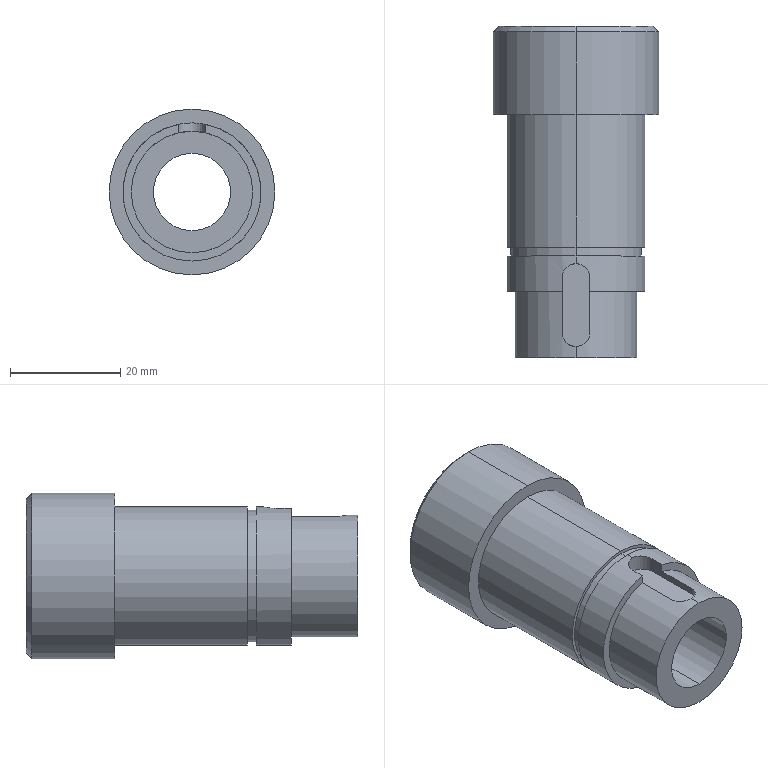Part | SolidWorks | features ICE 3, Chamfer 1, HoleWzd 1, RevCut 1, Revolution 1 | 1 solid | 28 faces | box 30 x 60 x 30 mm | volume 20081 mm3 | cylinder 16 | plane 10 | cone 2 | commonest cylinder face diameters 25 x4 5 x2 14 x2 18 x2 22 x2 23.8 x2
STEP:
#1=CARTESIAN_POINT('',(2.5,4.5,10.712));
#2=VERTEX_POINT('',#1);
#3=CARTESIAN_POINT('',(0.,2.,11.));
#4=VERTEX_POINT('',#3);
#5=CARTESIAN_POINT('',(2.5,4.5,10.712));
#6=CARTESIAN_POINT('',(2.5,4.334,10.712));
#7=CARTESIAN_POINT('',(2.484,4.171,10.716));
#8=CARTESIAN_POINT('',(2.42,3.851,10.731));
#9=CARTESIAN_POINT('',(2.371,3.692,10.742));
#10=CARTESIAN_POINT('',(2.246,3.389,10.769));
#11=CARTESIAN_POINT('',(2.169,3.246,10.784));
#12=CARTESIAN_POINT('',(1.987,2.974,10.819));
#13=CARTESIAN_POINT('',(1.882,2.846,10.838));
#14=CARTESIAN_POINT('',(1.537,2.502,10.895));
#15=CARTESIAN_POINT('',(1.259,2.316,10.932));
#16=CARTESIAN_POINT('',(0.8077,2.128,10.971));
#17=CARTESIAN_POINT('',(0.6494,2.08,10.982));
#18=CARTESIAN_POINT('',(0.3264,2.016,10.996));
#19=CARTESIAN_POINT('',(0.1637,2.,11.));
#20=CARTESIAN_POINT('',(0.,2.,11.));
#21=B_SPLINE_CURVE_WITH_KNOTS('',3,(#5,#6,#7,#8,#9,#10,#11,#12,#13,#14,#15,#16,#17,#18,#19,#20),.UNSPECIFIED.,.F.,.F.,(4,2,2,2,2,2,2,4),(0.,0.0004902,0.0009805,0.001471,0.001961,0.002941,0.003432,0.003922),.UNSPECIFIED.);
#22=EDGE_CURVE('',#2,#4,#21,.T.);
#23=ORIENTED_EDGE('',*,*,#22,.T.);
#24=CARTESIAN_POINT('',(0.,0.,11.));
#25=VERTEX_POINT('',#24);
#26=CARTESIAN_POINT('',(0.,12.,11.));
#27=DIRECTION('',(0.,-1.,0.));
#28=VECTOR('',#27,1000.);
#29=LINE('',#26,#28);
#30=EDGE_CURVE('',#4,#25,#29,.T.);
#31=ORIENTED_EDGE('',*,*,#30,.T.);
#32=CARTESIAN_POINT('',(0.,0.,-11.));
#33=VERTEX_POINT('',#32);
#34=CARTESIAN_POINT('',(0.,0.,0.));
#35=DIRECTION('',(0.,-1.,0.));
#36=DIRECTION('',(0.,0.,-1.));
#37=AXIS2_PLACEMENT_3D('',#34,#35,#36);
#38=CIRCLE('',#37,11.);
#39=EDGE_CURVE('',#33,#25,#38,.T.);
#40=ORIENTED_EDGE('',*,*,#39,.F.);
#41=CARTESIAN_POINT('',(0.,12.,-11.));
#42=VERTEX_POINT('',#41);
#43=CARTESIAN_POINT('',(0.,12.,-11.));
#44=DIRECTION('',(0.,-1.,0.));
#45=VECTOR('',#44,1000.);
#46=LINE('',#43,#45);
#47=EDGE_CURVE('',#42,#33,#46,.T.);
#48=ORIENTED_EDGE('',*,*,#47,.F.);
#49=CARTESIAN_POINT('',(2.5,12.,10.712));
#50=VERTEX_POINT('',#49);
#51=CARTESIAN_POINT('',(0.,12.,0.));
#52=DIRECTION('',(0.,-1.,0.));
#53=DIRECTION('',(0.,0.,-1.));
#54=AXIS2_PLACEMENT_3D('',#51,#52,#53);
#55=CIRCLE('',#54,11.);
#56=EDGE_CURVE('',#42,#50,#55,.T.);
#57=ORIENTED_EDGE('',*,*,#56,.T.);
#58=CARTESIAN_POINT('',(2.5,12.,10.712));
#59=DIRECTION('',(0.,-1.,0.));
#60=VECTOR('',#59,1000.);
#61=LINE('',#58,#60);
#62=EDGE_CURVE('',#50,#2,#61,.T.);
#63=ORIENTED_EDGE('',*,*,#62,.T.);
#64=EDGE_LOOP('',(#23,#31,#40,#48,#57,#63));
#65=FACE_OUTER_BOUND('',#64,.T.);
#66=CARTESIAN_POINT('',(0.,12.,0.));
#67=DIRECTION('',(0.,-1.,0.));
#68=DIRECTION('',(0.,0.,-1.));
#69=AXIS2_PLACEMENT_3D('',#66,#67,#68);
#70=CYLINDRICAL_SURFACE('',#69,11.);
#71=ADVANCED_FACE('',(#65),#70,.T.);
#72=CARTESIAN_POINT('',(0.,60.,14.));
#73=VERTEX_POINT('',#72);
#74=CARTESIAN_POINT('',(0.,60.,-14.));
#75=VERTEX_POINT('',#74);
#76=CARTESIAN_POINT('',(0.,60.,0.));
#77=DIRECTION('',(0.,1.,0.));
#78=DIRECTION('',(0.,0.,1.));
#79=AXIS2_PLACEMENT_3D('',#76,#77,#78);
#80=CIRCLE('',#79,14.);
#81=EDGE_CURVE('',#73,#75,#80,.T.);
#82=ORIENTED_EDGE('',*,*,#81,.F.);
#83=CARTESIAN_POINT('',(0.,59.,15.));
#84=VERTEX_POINT('',#83);
#85=CARTESIAN_POINT('',(0.,59.,15.));
#86=DIRECTION('',(0.,-0.7071,0.7071));
#87=VECTOR('',#86,1000.);
#88=LINE('',#85,#87);
#89=EDGE_CURVE('',#73,#84,#88,.T.);
#90=ORIENTED_EDGE('',*,*,#89,.T.);
#91=CARTESIAN_POINT('',(0.,59.,-15.));
#92=VERTEX_POINT('',#91);
#93=CARTESIAN_POINT('',(0.,59.,0.));
#94=DIRECTION('',(0.,-1.,0.));
#95=DIRECTION('',(0.,0.,1.));
#96=AXIS2_PLACEMENT_3D('',#93,#94,#95);
#97=CIRCLE('',#96,15.);
#98=EDGE_CURVE('',#92,#84,#97,.T.);
#99=ORIENTED_EDGE('',*,*,#98,.F.);
#100=CARTESIAN_POINT('',(0.,59.,-15.));
#101=DIRECTION('',(0.,-0.7071,-0.7071));
#102=VECTOR('',#101,1000.);
#103=LINE('',#100,#102);
#104=EDGE_CURVE('',#75,#92,#103,.T.);
#105=ORIENTED_EDGE('',*,*,#104,.F.);
#106=EDGE_LOOP('',(#82,#90,#99,#105));
#107=FACE_OUTER_BOUND('',#106,.T.);
#108=CARTESIAN_POINT('',(0.,59.,0.));
#109=DIRECTION('',(0.,-1.,0.));
#110=DIRECTION('',(0.,0.,-1.));
#111=AXIS2_PLACEMENT_3D('',#108,#109,#110);
#112=CONICAL_SURFACE('',#111,15.,0.7854);
#113=ADVANCED_FACE('',(#107),#112,.T.);
#114=CARTESIAN_POINT('',(0.,40.,-7.));
#115=VERTEX_POINT('',#114);
#116=CARTESIAN_POINT('',(0.,40.,7.));
#117=VERTEX_POINT('',#116);
#118=CARTESIAN_POINT('',(0.,40.,0.));
#119=DIRECTION('',(0.,1.,0.));
#120=DIRECTION('',(0.,0.,1.));
#121=AXIS2_PLACEMENT_3D('',#118,#119,#120);
#122=CIRCLE('',#121,7.);
#123=EDGE_CURVE('',#115,#117,#122,.T.);
#124=ORIENTED_EDGE('',*,*,#123,.T.);
#125=CARTESIAN_POINT('',(0.,0.,7.));
#126=VERTEX_POINT('',#125);
#127=CARTESIAN_POINT('',(0.,0.,7.));
#128=DIRECTION('',(0.,-1.,0.));
#129=VECTOR('',#128,1000.);
#130=LINE('',#127,#129);
#131=EDGE_CURVE('',#117,#126,#130,.T.);
#132=ORIENTED_EDGE('',*,*,#131,.T.);
#133=CARTESIAN_POINT('',(0.,0.,-7.));
#134=VERTEX_POINT('',#133);
#135=CARTESIAN_POINT('',(0.,0.,0.));
#136=DIRECTION('',(0.,-1.,0.));
#137=DIRECTION('',(0.,0.,-1.));
#138=AXIS2_PLACEMENT_3D('',#135,#136,#137);
#139=CIRCLE('',#138,7.);
#140=EDGE_CURVE('',#126,#134,#139,.T.);
#141=ORIENTED_EDGE('',*,*,#140,.T.);
#142=CARTESIAN_POINT('',(0.,0.,-7.));
#143=DIRECTION('',(0.,-1.,0.));
#144=VECTOR('',#143,1000.);
#145=LINE('',#142,#144);
#146=EDGE_CURVE('',#115,#134,#145,.T.);
#147=ORIENTED_EDGE('',*,*,#146,.F.);
#148=EDGE_LOOP('',(#124,#132,#141,#147));
#149=FACE_OUTER_BOUND('',#148,.T.);
#150=CARTESIAN_POINT('',(0.,0.,0.));
#151=DIRECTION('',(0.,-1.,0.));
#152=DIRECTION('',(0.,0.,-1.));
#153=AXIS2_PLACEMENT_3D('',#150,#151,#152);
#154=CYLINDRICAL_SURFACE('',#153,7.);
#155=ADVANCED_FACE('',(#149),#154,.F.);
#156=CARTESIAN_POINT('',(0.,40.,-9.));
#157=VERTEX_POINT('',#156);
#158=CARTESIAN_POINT('',(0.,40.,9.));
#159=VERTEX_POINT('',#158);
#160=CARTESIAN_POINT('',(0.,40.,0.));
#161=DIRECTION('',(0.,1.,0.));
#162=DIRECTION('',(0.,0.,1.));
#163=AXIS2_PLACEMENT_3D('',#160,#161,#162);
#164=CIRCLE('',#163,9.);
#165=EDGE_CURVE('',#157,#159,#164,.T.);
#166=ORIENTED_EDGE('',*,*,#165,.F.);
#167=CARTESIAN_POINT('',(0.,60.,-9.));
#168=VERTEX_POINT('',#167);
#169=CARTESIAN_POINT('',(0.,40.,-9.));
#170=DIRECTION('',(0.,1.,0.));
#171=VECTOR('',#170,1000.);
#172=LINE('',#169,#171);
#173=EDGE_CURVE('',#157,#168,#172,.T.);
#174=ORIENTED_EDGE('',*,*,#173,.T.);
#175=CARTESIAN_POINT('',(0.,60.,9.));
#176=VERTEX_POINT('',#175);
#177=CARTESIAN_POINT('',(0.,60.,0.));
#178=DIRECTION('',(0.,1.,0.));
#179=DIRECTION('',(0.,0.,1.));
#180=AXIS2_PLACEMENT_3D('',#177,#178,#179);
#181=CIRCLE('',#180,9.);
#182=EDGE_CURVE('',#168,#176,#181,.T.);
#183=ORIENTED_EDGE('',*,*,#182,.T.);
#184=CARTESIAN_POINT('',(0.,40.,9.));
#185=DIRECTION('',(0.,1.,0.));
#186=VECTOR('',#185,1000.);
#187=LINE('',#184,#186);
#188=EDGE_CURVE('',#159,#176,#187,.T.);
#189=ORIENTED_EDGE('',*,*,#188,.F.);
#190=EDGE_LOOP('',(#166,#174,#183,#189));
#191=FACE_OUTER_BOUND('',#190,.T.);
#192=CARTESIAN_POINT('',(0.,40.,0.));
#193=DIRECTION('',(0.,1.,0.));
#194=DIRECTION('',(0.,0.,1.));
#195=AXIS2_PLACEMENT_3D('',#192,#193,#194);
#196=CYLINDRICAL_SURFACE('',#195,9.);
#197=ADVANCED_FACE('',(#191),#196,.F.);
#198=CARTESIAN_POINT('',(0.,20.,-11.9));
#199=VERTEX_POINT('',#198);
#200=CARTESIAN_POINT('',(0.,20.,11.9));
#201=VERTEX_POINT('',#200);
#202=CARTESIAN_POINT('',(0.,20.,0.));
#203=DIRECTION('',(0.,-1.,0.));
#204=DIRECTION('',(0.,0.,-1.));
#205=AXIS2_PLACEMENT_3D('',#202,#203,#204);
#206=CIRCLE('',#205,11.9);
#207=EDGE_CURVE('',#199,#201,#206,.T.);
#208=ORIENTED_EDGE('',*,*,#207,.T.);
#209=CARTESIAN_POINT('',(0.,18.4,11.9));
#210=VERTEX_POINT('',#209);
#211=CARTESIAN_POINT('',(0.,0.,11.9));
#212=DIRECTION('',(0.,-1.,0.));
#213=VECTOR('',#212,1000.);
#214=LINE('',#211,#213);
#215=EDGE_CURVE('',#201,#210,#214,.T.);
#216=ORIENTED_EDGE('',*,*,#215,.T.);
#217=CARTESIAN_POINT('',(0.,18.4,-11.9));
#218=VERTEX_POINT('',#217);
#219=CARTESIAN_POINT('',(0.,18.4,0.));
#220=DIRECTION('',(0.,-1.,0.));
#221=DIRECTION('',(0.,0.,-1.));
#222=AXIS2_PLACEMENT_3D('',#219,#220,#221);
#223=CIRCLE('',#222,11.9);
#224=EDGE_CURVE('',#218,#210,#223,.T.);
#225=ORIENTED_EDGE('',*,*,#224,.F.);
#226=CARTESIAN_POINT('',(0.,0.,-11.9));
#227=DIRECTION('',(0.,-1.,0.));
#228=VECTOR('',#227,1000.);
#229=LINE('',#226,#228);
#230=EDGE_CURVE('',#199,#218,#229,.T.);
#231=ORIENTED_EDGE('',*,*,#230,.F.);
#232=EDGE_LOOP('',(#208,#216,#225,#231));
#233=FACE_OUTER_BOUND('',#232,.T.);
#234=CARTESIAN_POINT('',(0.,0.,0.));
#235=DIRECTION('',(0.,-1.,0.));
#236=DIRECTION('',(0.,0.,-1.));
#237=AXIS2_PLACEMENT_3D('',#234,#235,#236);
#238=CYLINDRICAL_SURFACE('',#237,11.9);
#239=ADVANCED_FACE('',(#233),#238,.T.);
#240=ORIENTED_EDGE('',*,*,#98,.T.);
#241=CARTESIAN_POINT('',(0.,44.,15.));
#242=VERTEX_POINT('',#241);
#243=CARTESIAN_POINT('',(0.,0.,15.));
#244=DIRECTION('',(0.,-1.,0.));
#245=VECTOR('',#244,1000.);
#246=LINE('',#243,#245);
#247=EDGE_CURVE('',#84,#242,#246,.T.);
#248=ORIENTED_EDGE('',*,*,#247,.T.);
#249=CARTESIAN_POINT('',(0.,44.,-15.));
#250=VERTEX_POINT('',#249);
#251=CARTESIAN_POINT('',(0.,44.,0.));
#252=DIRECTION('',(0.,-1.,0.));
#253=DIRECTION('',(0.,0.,-1.));
#254=AXIS2_PLACEMENT_3D('',#251,#252,#253);
#255=CIRCLE('',#254,15.);
#256=EDGE_CURVE('',#250,#242,#255,.T.);
#257=ORIENTED_EDGE('',*,*,#256,.F.);
#258=CARTESIAN_POINT('',(0.,0.,-15.));
#259=DIRECTION('',(0.,-1.,0.));
#260=VECTOR('',#259,1000.);
#261=LINE('',#258,#260);
#262=EDGE_CURVE('',#92,#250,#261,.T.);
#263=ORIENTED_EDGE('',*,*,#262,.F.);
#264=EDGE_LOOP('',(#240,#248,#257,#263));
#265=FACE_OUTER_BOUND('',#264,.T.);
#266=CARTESIAN_POINT('',(0.,0.,0.));
#267=DIRECTION('',(0.,-1.,0.));
#268=DIRECTION('',(0.,0.,-1.));
#269=AXIS2_PLACEMENT_3D('',#266,#267,#268);
#270=CYLINDRICAL_SURFACE('',#269,15.);
#271=ADVANCED_FACE('',(#265),#270,.T.);
#272=CARTESIAN_POINT('',(0.,44.,-12.5));
#273=VERTEX_POINT('',#272);
#274=CARTESIAN_POINT('',(0.,44.,12.5));
#275=VERTEX_POINT('',#274);
#276=CARTESIAN_POINT('',(0.,44.,0.));
#277=DIRECTION('',(0.,-1.,0.));
#278=DIRECTION('',(0.,0.,-1.));
#279=AXIS2_PLACEMENT_3D('',#276,#277,#278);
#280=CIRCLE('',#279,12.5);
#281=EDGE_CURVE('',#273,#275,#280,.T.);
#282=ORIENTED_EDGE('',*,*,#281,.T.);
#283=CARTESIAN_POINT('',(0.,20.,12.5));
#284=VERTEX_POINT('',#283);
#285=CARTESIAN_POINT('',(0.,0.,12.5));
#286=DIRECTION('',(0.,-1.,0.));
#287=VECTOR('',#286,1000.);
#288=LINE('',#285,#287);
#289=EDGE_CURVE('',#275,#284,#288,.T.);
#290=ORIENTED_EDGE('',*,*,#289,.T.);
#291=CARTESIAN_POINT('',(0.,20.,-12.5));
#292=VERTEX_POINT('',#291);
#293=CARTESIAN_POINT('',(0.,20.,0.));
#294=DIRECTION('',(0.,1.,0.));
#295=DIRECTION('',(0.,0.,-1.));
#296=AXIS2_PLACEMENT_3D('',#293,#294,#295);
#297=CIRCLE('',#296,12.5);
#298=EDGE_CURVE('',#284,#292,#297,.T.);
#299=ORIENTED_EDGE('',*,*,#298,.T.);
#300=CARTESIAN_POINT('',(0.,0.,-12.5));
#301=DIRECTION('',(0.,-1.,0.));
#302=VECTOR('',#301,1000.);
#303=LINE('',#300,#302);
#304=EDGE_CURVE('',#273,#292,#303,.T.);
#305=ORIENTED_EDGE('',*,*,#304,.F.);
#306=EDGE_LOOP('',(#282,#290,#299,#305));
#307=FACE_OUTER_BOUND('',#306,.T.);
#308=CARTESIAN_POINT('',(0.,0.,0.));
#309=DIRECTION('',(0.,-1.,0.));
#310=DIRECTION('',(0.,0.,-1.));
#311=AXIS2_PLACEMENT_3D('',#308,#309,#310);
#312=CYLINDRICAL_SURFACE('',#311,12.5);
#313=ADVANCED_FACE('',(#307),#312,.T.);
#314=CARTESIAN_POINT('',(0.,18.4,-12.5));
#315=VERTEX_POINT('',#314);
#316=CARTESIAN_POINT('',(0.,18.4,12.5));
#317=VERTEX_POINT('',#316);
#318=CARTESIAN_POINT('',(0.,18.4,0.));
#319=DIRECTION('',(0.,-1.,0.));
#320=DIRECTION('',(0.,0.,1.));
#321=AXIS2_PLACEMENT_3D('',#318,#319,#320);
#322=CIRCLE('',#321,12.5);
#323=EDGE_CURVE('',#315,#317,#322,.T.);
#324=ORIENTED_EDGE('',*,*,#323,.T.);
#325=CARTESIAN_POINT('',(0.,17.,12.5));
#326=VERTEX_POINT('',#325);
#327=CARTESIAN_POINT('',(0.,0.,12.5));
#328=DIRECTION('',(0.,-1.,0.));
#329=VECTOR('',#328,1000.);
#330=LINE('',#327,#329);
#331=EDGE_CURVE('',#317,#326,#330,.T.);
#332=ORIENTED_EDGE('',*,*,#331,.T.);
#333=CARTESIAN_POINT('',(2.5,14.5,12.247));
#334=VERTEX_POINT('',#333);
#335=CARTESIAN_POINT('',(2.5,14.5,12.247));
#336=CARTESIAN_POINT('',(2.5,14.666,12.247));
#337=CARTESIAN_POINT('',(2.484,14.828,12.251));
#338=CARTESIAN_POINT('',(2.42,15.149,12.264));
#339=CARTESIAN_POINT('',(2.372,15.308,12.273));
#340=CARTESIAN_POINT('',(2.246,15.61,12.297));
#341=CARTESIAN_POINT('',(2.169,15.754,12.311));
#342=CARTESIAN_POINT('',(1.987,16.025,12.341));
#343=CARTESIAN_POINT('',(1.882,16.154,12.358));
#344=CARTESIAN_POINT('',(1.537,16.498,12.407));
#345=CARTESIAN_POINT('',(1.258,16.685,12.44));
#346=CARTESIAN_POINT('',(0.8073,16.872,12.475));
#347=CARTESIAN_POINT('',(0.6491,16.92,12.484));
#348=CARTESIAN_POINT('',(0.3261,16.984,12.497));
#349=CARTESIAN_POINT('',(0.1636,17.,12.5));
#350=CARTESIAN_POINT('',(0.,17.,12.5));
#351=B_SPLINE_CURVE_WITH_KNOTS('',3,(#335,#336,#337,#338,#339,#340,#341,#342,#343,#344,#345,#346,#347,#348,#349,#350),.UNSPECIFIED.,.F.,.F.,(4,2,2,2,2,2,2,4),(0.,0.0004899,0.0009797,0.00147,0.001959,0.002939,0.003429,0.003919),.UNSPECIFIED.);
#352=EDGE_CURVE('',#334,#326,#351,.T.);
#353=ORIENTED_EDGE('',*,*,#352,.F.);
#354=CARTESIAN_POINT('',(2.5,12.,12.247));
#355=VERTEX_POINT('',#354);
#356=CARTESIAN_POINT('',(2.5,0.,12.247));
#357=DIRECTION('',(0.,1.,0.));
#358=VECTOR('',#357,1000.);
#359=LINE('',#356,#358);
#360=EDGE_CURVE('',#355,#334,#359,.T.);
#361=ORIENTED_EDGE('',*,*,#360,.F.);
#362=CARTESIAN_POINT('',(0.,12.,-12.5));
#363=VERTEX_POINT('',#362);
#364=CARTESIAN_POINT('',(0.,12.,0.));
#365=DIRECTION('',(0.,1.,0.));
#366=DIRECTION('',(0.,0.,-1.));
#367=AXIS2_PLACEMENT_3D('',#364,#365,#366);
#368=CIRCLE('',#367,12.5);
#369=EDGE_CURVE('',#355,#363,#368,.T.);
#370=ORIENTED_EDGE('',*,*,#369,.T.);
#371=CARTESIAN_POINT('',(0.,0.,-12.5));
#372=DIRECTION('',(0.,-1.,0.));
#373=VECTOR('',#372,1000.);
#374=LINE('',#371,#373);
#375=EDGE_CURVE('',#315,#363,#374,.T.);
#376=ORIENTED_EDGE('',*,*,#375,.F.);
#377=EDGE_LOOP('',(#324,#332,#353,#361,#370,#376));
#378=FACE_OUTER_BOUND('',#377,.T.);
#379=CARTESIAN_POINT('',(0.,0.,0.));
#380=DIRECTION('',(0.,-1.,0.));
#381=DIRECTION('',(0.,0.,-1.));
#382=AXIS2_PLACEMENT_3D('',#379,#380,#381);
#383=CYLINDRICAL_SURFACE('',#382,12.5);
#384=ADVANCED_FACE('',(#378),#383,.T.);
#385=ORIENTED_EDGE('',*,*,#331,.F.);
#386=CARTESIAN_POINT('',(0.,18.4,0.));
#387=DIRECTION('',(0.,-1.,0.));
#388=DIRECTION('',(0.,0.,1.));
#389=AXIS2_PLACEMENT_3D('',#386,#387,#388);
#390=CIRCLE('',#389,12.5);
#391=EDGE_CURVE('',#317,#315,#390,.T.);
#392=ORIENTED_EDGE('',*,*,#391,.T.);
#393=ORIENTED_EDGE('',*,*,#375,.T.);
#394=CARTESIAN_POINT('',(-2.5,12.,12.247));
#395=VERTEX_POINT('',#394);
#396=CARTESIAN_POINT('',(0.,12.,0.));
#397=DIRECTION('',(0.,1.,0.));
#398=DIRECTION('',(0.,0.,-1.));
#399=AXIS2_PLACEMENT_3D('',#396,#397,#398);
#400=CIRCLE('',#399,12.5);
#401=EDGE_CURVE('',#363,#395,#400,.T.);
#402=ORIENTED_EDGE('',*,*,#401,.T.);
#403=CARTESIAN_POINT('',(-2.5,14.5,12.247));
#404=VERTEX_POINT('',#403);
#405=CARTESIAN_POINT('',(-2.5,0.,12.247));
#406=DIRECTION('',(0.,-1.,0.));
#407=VECTOR('',#406,1000.);
#408=LINE('',#405,#407);
#409=EDGE_CURVE('',#404,#395,#408,.T.);
#410=ORIENTED_EDGE('',*,*,#409,.F.);
#411=CARTESIAN_POINT('',(0.,17.,12.5));
#412=CARTESIAN_POINT('',(-0.1634,17.,12.5));
#413=CARTESIAN_POINT('',(-0.3294,16.984,12.497));
#414=CARTESIAN_POINT('',(-0.6501,16.92,12.484));
#415=CARTESIAN_POINT('',(-0.806,16.872,12.475));
#416=CARTESIAN_POINT('',(-1.109,16.747,12.452));
#417=CARTESIAN_POINT('',(-1.255,16.668,12.438));
#418=CARTESIAN_POINT('',(-1.525,16.488,12.407));
#419=CARTESIAN_POINT('',(-1.651,16.384,12.391));
#420=CARTESIAN_POINT('',(-1.884,16.152,12.358));
#421=CARTESIAN_POINT('',(-1.987,16.026,12.341));
#422=CARTESIAN_POINT('',(-2.168,15.756,12.311));
#423=CARTESIAN_POINT('',(-2.246,15.61,12.297));
#424=CARTESIAN_POINT('',(-2.371,15.308,12.273));
#425=CARTESIAN_POINT('',(-2.419,15.152,12.264));
#426=CARTESIAN_POINT('',(-2.483,14.831,12.251));
#427=CARTESIAN_POINT('',(-2.5,14.666,12.247));
#428=CARTESIAN_POINT('',(-2.5,14.5,12.247));
#429=B_SPLINE_CURVE_WITH_KNOTS('',3,(#411,#412,#413,#414,#415,#416,#417,#418,#419,#420,#421,#422,#423,#424,#425,#426,#427,#428),.UNSPECIFIED.,.F.,.F.,(4,2,2,2,2,2,2,2,4),(0.003919,0.004408,0.004898,0.005387,0.005876,0.006366,0.006855,0.007344,0.007834),.UNSPECIFIED.);
#430=EDGE_CURVE('',#326,#404,#429,.T.);
#431=ORIENTED_EDGE('',*,*,#430,.F.);
#432=EDGE_LOOP('',(#385,#392,#393,#402,#410,#431));
#433=FACE_OUTER_BOUND('',#432,.T.);
#434=CARTESIAN_POINT('',(0.,0.,0.));
#435=DIRECTION('',(0.,-1.,0.));
#436=DIRECTION('',(0.,0.,-1.));
#437=AXIS2_PLACEMENT_3D('',#434,#435,#436);
#438=CYLINDRICAL_SURFACE('',#437,12.5);
#439=ADVANCED_FACE('',(#433),#438,.T.);
#440=CARTESIAN_POINT('',(0.,0.,0.));
#441=DIRECTION('',(0.,-1.,0.));
#442=DIRECTION('',(0.,0.,-1.));
#443=AXIS2_PLACEMENT_3D('',#440,#441,#442);
#444=CIRCLE('',#443,7.);
#445=EDGE_CURVE('',#134,#126,#444,.T.);
#446=ORIENTED_EDGE('',*,*,#445,.F.);
#447=ORIENTED_EDGE('',*,*,#140,.F.);
#448=EDGE_LOOP('',(#446,#447));
#449=FACE_BOUND('',#448,.T.);
#450=ORIENTED_EDGE('',*,*,#39,.T.);
#451=CARTESIAN_POINT('',(0.,0.,0.));
#452=DIRECTION('',(0.,-1.,0.));
#453=DIRECTION('',(0.,0.,-1.));
#454=AXIS2_PLACEMENT_3D('',#451,#452,#453);
#455=CIRCLE('',#454,11.);
#456=EDGE_CURVE('',#25,#33,#455,.T.);
#457=ORIENTED_EDGE('',*,*,#456,.T.);
#458=EDGE_LOOP('',(#450,#457));
#459=FACE_OUTER_BOUND('',#458,.T.);
#460=CARTESIAN_POINT('',(12.5,0.,0.));
#461=DIRECTION('',(0.,-1.,0.));
#462=DIRECTION('',(0.,0.,-1.));
#463=AXIS2_PLACEMENT_3D('',#460,#461,#462);
#464=PLANE('',#463);
#465=ADVANCED_FACE('',(#449,#459),#464,.T.);
#466=CARTESIAN_POINT('',(2.5,12.,9.5));
#467=DIRECTION('',(0.,0.,-1.));
#468=VECTOR('',#467,1000.);
#469=LINE('',#466,#468);
#470=EDGE_CURVE('',#355,#50,#469,.T.);
#471=ORIENTED_EDGE('',*,*,#470,.F.);
#472=ORIENTED_EDGE('',*,*,#360,.T.);
#473=CARTESIAN_POINT('',(2.5,14.5,9.5));
#474=VERTEX_POINT('',#473);
#475=CARTESIAN_POINT('',(2.5,14.5,9.5));
#476=DIRECTION('',(0.,0.,1.));
#477=VECTOR('',#476,1000.);
#478=LINE('',#475,#477);
#479=EDGE_CURVE('',#474,#334,#478,.T.);
#480=ORIENTED_EDGE('',*,*,#479,.F.);
#481=CARTESIAN_POINT('',(2.5,4.5,9.5));
#482=VERTEX_POINT('',#481);
#483=CARTESIAN_POINT('',(2.5,14.5,9.5));
#484=DIRECTION('',(0.,1.,0.));
#485=VECTOR('',#484,1000.);
#486=LINE('',#483,#485);
#487=EDGE_CURVE('',#482,#474,#486,.T.);
#488=ORIENTED_EDGE('',*,*,#487,.F.);
#489=CARTESIAN_POINT('',(2.5,4.5,9.5));
#490=DIRECTION('',(0.,0.,1.));
#491=VECTOR('',#490,1000.);
#492=LINE('',#489,#491);
#493=EDGE_CURVE('',#482,#2,#492,.T.);
#494=ORIENTED_EDGE('',*,*,#493,.T.);
#495=ORIENTED_EDGE('',*,*,#62,.F.);
#496=EDGE_LOOP('',(#471,#472,#480,#488,#494,#495));
#497=FACE_OUTER_BOUND('',#496,.T.);
#498=CARTESIAN_POINT('',(2.5,14.5,9.5));
#499=DIRECTION('',(1.,0.,0.));
#500=DIRECTION('',(0.,1.,0.));
#501=AXIS2_PLACEMENT_3D('',#498,#499,#500);
#502=PLANE('',#501);
#503=ADVANCED_FACE('',(#497),#502,.F.);
#504=ORIENTED_EDGE('',*,*,#22,.F.);
#505=ORIENTED_EDGE('',*,*,#493,.F.);
#506=CARTESIAN_POINT('',(-2.5,4.5,9.5));
#507=VERTEX_POINT('',#506);
#508=CARTESIAN_POINT('',(0.,4.5,9.5));
#509=DIRECTION('',(0.,0.,1.));
#510=DIRECTION('',(1.,0.,0.));
#511=AXIS2_PLACEMENT_3D('',#508,#509,#510);
#512=CIRCLE('',#511,2.5);
#513=EDGE_CURVE('',#507,#482,#512,.T.);
#514=ORIENTED_EDGE('',*,*,#513,.F.);
#515=CARTESIAN_POINT('',(-2.5,4.5,10.712));
#516=VERTEX_POINT('',#515);
#517=CARTESIAN_POINT('',(-2.5,4.5,9.5));
#518=DIRECTION('',(0.,0.,1.));
#519=VECTOR('',#518,1000.);
#520=LINE('',#517,#519);
#521=EDGE_CURVE('',#507,#516,#520,.T.);
#522=ORIENTED_EDGE('',*,*,#521,.T.);
#523=CARTESIAN_POINT('',(0.,2.,11.));
#524=CARTESIAN_POINT('',(-0.1635,2.,11.));
#525=CARTESIAN_POINT('',(-0.3297,2.016,10.996));
#526=CARTESIAN_POINT('',(-0.6505,2.081,10.982));
#527=CARTESIAN_POINT('',(-0.8065,2.128,10.971));
#528=CARTESIAN_POINT('',(-1.261,2.317,10.932));
#529=CARTESIAN_POINT('',(-1.536,2.5,10.895));
#530=CARTESIAN_POINT('',(-1.884,2.848,10.838));
#531=CARTESIAN_POINT('',(-1.987,2.974,10.82));
#532=CARTESIAN_POINT('',(-2.167,3.244,10.785));
#533=CARTESIAN_POINT('',(-2.246,3.39,10.768));
#534=CARTESIAN_POINT('',(-2.371,3.692,10.742));
#535=CARTESIAN_POINT('',(-2.419,3.847,10.731));
#536=CARTESIAN_POINT('',(-2.483,4.169,10.716));
#537=CARTESIAN_POINT('',(-2.5,4.334,10.712));
#538=CARTESIAN_POINT('',(-2.5,4.5,10.712));
#539=B_SPLINE_CURVE_WITH_KNOTS('',3,(#523,#524,#525,#526,#527,#528,#529,#530,#531,#532,#533,#534,#535,#536,#537,#538),.UNSPECIFIED.,.F.,.F.,(4,2,2,2,2,2,2,4),(0.003922,0.004412,0.004901,0.005881,0.00637,0.00686,0.00735,0.00784),.UNSPECIFIED.);
#540=EDGE_CURVE('',#4,#516,#539,.T.);
#541=ORIENTED_EDGE('',*,*,#540,.F.);
#542=EDGE_LOOP('',(#504,#505,#514,#522,#541));
#543=FACE_OUTER_BOUND('',#542,.T.);
#544=CARTESIAN_POINT('',(0.,4.5,9.5));
#545=DIRECTION('',(0.,0.,1.));
#546=DIRECTION('',(1.,0.,0.));
#547=AXIS2_PLACEMENT_3D('',#544,#545,#546);
#548=CYLINDRICAL_SURFACE('',#547,2.5);
#549=ADVANCED_FACE('',(#543),#548,.F.);
#550=CARTESIAN_POINT('',(-2.5,12.,10.712));
#551=VERTEX_POINT('',#550);
#552=CARTESIAN_POINT('',(-2.5,12.,9.5));
#553=DIRECTION('',(0.,0.,1.));
#554=VECTOR('',#553,1000.);
#555=LINE('',#552,#554);
#556=EDGE_CURVE('',#551,#395,#555,.T.);
#557=ORIENTED_EDGE('',*,*,#556,.F.);
#558=CARTESIAN_POINT('',(-2.5,12.,10.712));
#559=DIRECTION('',(0.,1.,0.));
#560=VECTOR('',#559,1000.);
#561=LINE('',#558,#560);
#562=EDGE_CURVE('',#516,#551,#561,.T.);
#563=ORIENTED_EDGE('',*,*,#562,.F.);
#564=ORIENTED_EDGE('',*,*,#521,.F.);
#565=CARTESIAN_POINT('',(-2.5,14.5,9.5));
#566=VERTEX_POINT('',#565);
#567=CARTESIAN_POINT('',(-2.5,14.5,9.5));
#568=DIRECTION('',(0.,-1.,0.));
#569=VECTOR('',#568,1000.);
#570=LINE('',#567,#569);
#571=EDGE_CURVE('',#566,#507,#570,.T.);
#572=ORIENTED_EDGE('',*,*,#571,.F.);
#573=CARTESIAN_POINT('',(-2.5,14.5,9.5));
#574=DIRECTION('',(0.,0.,1.));
#575=VECTOR('',#574,1000.);
#576=LINE('',#573,#575);
#577=EDGE_CURVE('',#566,#404,#576,.T.);
#578=ORIENTED_EDGE('',*,*,#577,.T.);
#579=ORIENTED_EDGE('',*,*,#409,.T.);
#580=EDGE_LOOP('',(#557,#563,#564,#572,#578,#579));
#581=FACE_OUTER_BOUND('',#580,.T.);
#582=CARTESIAN_POINT('',(-2.5,14.5,9.5));
#583=DIRECTION('',(-1.,0.,0.));
#584=DIRECTION('',(0.,-1.,0.));
#585=AXIS2_PLACEMENT_3D('',#582,#583,#584);
#586=PLANE('',#585);
#587=ADVANCED_FACE('',(#581),#586,.F.);
#588=ORIENTED_EDGE('',*,*,#289,.F.);
#589=CARTESIAN_POINT('',(0.,44.,0.));
#590=DIRECTION('',(0.,-1.,0.));
#591=DIRECTION('',(0.,0.,-1.));
#592=AXIS2_PLACEMENT_3D('',#589,#590,#591);
#593=CIRCLE('',#592,12.5);
#594=EDGE_CURVE('',#275,#273,#593,.T.);
#595=ORIENTED_EDGE('',*,*,#594,.T.);
#596=ORIENTED_EDGE('',*,*,#304,.T.);
#597=CARTESIAN_POINT('',(0.,20.,0.));
#598=DIRECTION('',(0.,1.,0.));
#599=DIRECTION('',(0.,0.,-1.));
#600=AXIS2_PLACEMENT_3D('',#597,#598,#599);
#601=CIRCLE('',#600,12.5);
#602=EDGE_CURVE('',#292,#284,#601,.T.);
#603=ORIENTED_EDGE('',*,*,#602,.T.);
#604=EDGE_LOOP('',(#588,#595,#596,#603));
#605=FACE_OUTER_BOUND('',#604,.T.);
#606=CARTESIAN_POINT('',(0.,0.,0.));
#607=DIRECTION('',(0.,-1.,0.));
#608=DIRECTION('',(0.,0.,-1.));
#609=AXIS2_PLACEMENT_3D('',#606,#607,#608);
#610=CYLINDRICAL_SURFACE('',#609,12.5);
#611=ADVANCED_FACE('',(#605),#610,.T.);
#612=ORIENTED_EDGE('',*,*,#256,.T.);
#613=CARTESIAN_POINT('',(0.,44.,0.));
#614=DIRECTION('',(0.,-1.,0.));
#615=DIRECTION('',(0.,0.,-1.));
#616=AXIS2_PLACEMENT_3D('',#613,#614,#615);
#617=CIRCLE('',#616,15.);
#618=EDGE_CURVE('',#242,#250,#617,.T.);
#619=ORIENTED_EDGE('',*,*,#618,.T.);
#620=EDGE_LOOP('',(#612,#619));
#621=FACE_OUTER_BOUND('',#620,.T.);
#622=ORIENTED_EDGE('',*,*,#281,.F.);
#623=ORIENTED_EDGE('',*,*,#594,.F.);
#624=EDGE_LOOP('',(#622,#623));
#625=FACE_BOUND('',#624,.T.);
#626=CARTESIAN_POINT('',(15.,44.,0.));
#627=DIRECTION('',(0.,-1.,0.));
#628=DIRECTION('',(0.,0.,-1.));
#629=AXIS2_PLACEMENT_3D('',#626,#627,#628);
#630=PLANE('',#629);
#631=ADVANCED_FACE('',(#621,#625),#630,.T.);
#632=ORIENTED_EDGE('',*,*,#247,.F.);
#633=CARTESIAN_POINT('',(0.,59.,0.));
#634=DIRECTION('',(0.,-1.,0.));
#635=DIRECTION('',(0.,0.,1.));
#636=AXIS2_PLACEMENT_3D('',#633,#634,#635);
#637=CIRCLE('',#636,15.);
#638=EDGE_CURVE('',#84,#92,#637,.T.);
#639=ORIENTED_EDGE('',*,*,#638,.T.);
#640=ORIENTED_EDGE('',*,*,#262,.T.);
#641=ORIENTED_EDGE('',*,*,#618,.F.);
#642=EDGE_LOOP('',(#632,#639,#640,#641));
#643=FACE_OUTER_BOUND('',#642,.T.);
#644=CARTESIAN_POINT('',(0.,0.,0.));
#645=DIRECTION('',(0.,-1.,0.));
#646=DIRECTION('',(0.,0.,-1.));
#647=AXIS2_PLACEMENT_3D('',#644,#645,#646);
#648=CYLINDRICAL_SURFACE('',#647,15.);
#649=ADVANCED_FACE('',(#643),#648,.T.);
#650=CARTESIAN_POINT('',(0.,60.,0.));
#651=DIRECTION('',(0.,1.,0.));
#652=DIRECTION('',(0.,0.,1.));
#653=AXIS2_PLACEMENT_3D('',#650,#651,#652);
#654=CIRCLE('',#653,14.);
#655=EDGE_CURVE('',#75,#73,#654,.T.);
#656=ORIENTED_EDGE('',*,*,#655,.T.);
#657=ORIENTED_EDGE('',*,*,#81,.T.);
#658=EDGE_LOOP('',(#656,#657));
#659=FACE_OUTER_BOUND('',#658,.T.);
#660=CARTESIAN_POINT('',(0.,60.,0.));
#661=DIRECTION('',(0.,1.,0.));
#662=DIRECTION('',(0.,0.,1.));
#663=AXIS2_PLACEMENT_3D('',#660,#661,#662);
#664=CIRCLE('',#663,9.);
#665=EDGE_CURVE('',#176,#168,#664,.T.);
#666=ORIENTED_EDGE('',*,*,#665,.F.);
#667=ORIENTED_EDGE('',*,*,#182,.F.);
#668=EDGE_LOOP('',(#666,#667));
#669=FACE_BOUND('',#668,.T.);
#670=CARTESIAN_POINT('',(6.,60.,0.));
#671=DIRECTION('',(0.,1.,0.));
#672=DIRECTION('',(0.,0.,1.));
#673=AXIS2_PLACEMENT_3D('',#670,#671,#672);
#674=PLANE('',#673);
#675=ADVANCED_FACE('',(#659,#669),#674,.T.);
#676=ORIENTED_EDGE('',*,*,#323,.F.);
#677=ORIENTED_EDGE('',*,*,#391,.F.);
#678=EDGE_LOOP('',(#676,#677));
#679=FACE_OUTER_BOUND('',#678,.T.);
#680=ORIENTED_EDGE('',*,*,#224,.T.);
#681=CARTESIAN_POINT('',(0.,18.4,0.));
#682=DIRECTION('',(0.,-1.,0.));
#683=DIRECTION('',(0.,0.,-1.));
#684=AXIS2_PLACEMENT_3D('',#681,#682,#683);
#685=CIRCLE('',#684,11.9);
#686=EDGE_CURVE('',#210,#218,#685,.T.);
#687=ORIENTED_EDGE('',*,*,#686,.T.);
#688=EDGE_LOOP('',(#680,#687));
#689=FACE_BOUND('',#688,.T.);
#690=CARTESIAN_POINT('',(-16.774,18.4,0.));
#691=DIRECTION('',(0.,1.,0.));
#692=DIRECTION('',(0.,0.,1.));
#693=AXIS2_PLACEMENT_3D('',#690,#691,#692);
#694=PLANE('',#693);
#695=ADVANCED_FACE('',(#679,#689),#694,.T.);
#696=ORIENTED_EDGE('',*,*,#215,.F.);
#697=CARTESIAN_POINT('',(0.,20.,0.));
#698=DIRECTION('',(0.,-1.,0.));
#699=DIRECTION('',(0.,0.,-1.));
#700=AXIS2_PLACEMENT_3D('',#697,#698,#699);
#701=CIRCLE('',#700,11.9);
#702=EDGE_CURVE('',#201,#199,#701,.T.);
#703=ORIENTED_EDGE('',*,*,#702,.T.);
#704=ORIENTED_EDGE('',*,*,#230,.T.);
#705=ORIENTED_EDGE('',*,*,#686,.F.);
#706=EDGE_LOOP('',(#696,#703,#704,#705));
#707=FACE_OUTER_BOUND('',#706,.T.);
#708=CARTESIAN_POINT('',(0.,0.,0.));
#709=DIRECTION('',(0.,-1.,0.));
#710=DIRECTION('',(0.,0.,-1.));
#711=AXIS2_PLACEMENT_3D('',#708,#709,#710);
#712=CYLINDRICAL_SURFACE('',#711,11.9);
#713=ADVANCED_FACE('',(#707),#712,.T.);
#714=ORIENTED_EDGE('',*,*,#602,.F.);
#715=ORIENTED_EDGE('',*,*,#298,.F.);
#716=EDGE_LOOP('',(#714,#715));
#717=FACE_OUTER_BOUND('',#716,.T.);
#718=ORIENTED_EDGE('',*,*,#207,.F.);
#719=ORIENTED_EDGE('',*,*,#702,.F.);
#720=EDGE_LOOP('',(#718,#719));
#721=FACE_BOUND('',#720,.T.);
#722=CARTESIAN_POINT('',(-16.774,20.,0.));
#723=DIRECTION('',(0.,-1.,0.));
#724=DIRECTION('',(0.,0.,-1.));
#725=AXIS2_PLACEMENT_3D('',#722,#723,#724);
#726=PLANE('',#725);
#727=ADVANCED_FACE('',(#717,#721),#726,.T.);
#728=ORIENTED_EDGE('',*,*,#173,.F.);
#729=CARTESIAN_POINT('',(0.,40.,0.));
#730=DIRECTION('',(0.,1.,0.));
#731=DIRECTION('',(0.,0.,1.));
#732=AXIS2_PLACEMENT_3D('',#729,#730,#731);
#733=CIRCLE('',#732,9.);
#734=EDGE_CURVE('',#159,#157,#733,.T.);
#735=ORIENTED_EDGE('',*,*,#734,.F.);
#736=ORIENTED_EDGE('',*,*,#188,.T.);
#737=ORIENTED_EDGE('',*,*,#665,.T.);
#738=EDGE_LOOP('',(#728,#735,#736,#737));
#739=FACE_OUTER_BOUND('',#738,.T.);
#740=CARTESIAN_POINT('',(0.,40.,0.));
#741=DIRECTION('',(0.,1.,0.));
#742=DIRECTION('',(0.,0.,1.));
#743=AXIS2_PLACEMENT_3D('',#740,#741,#742);
#744=CYLINDRICAL_SURFACE('',#743,9.);
#745=ADVANCED_FACE('',(#739),#744,.F.);
#746=ORIENTED_EDGE('',*,*,#123,.F.);
#747=CARTESIAN_POINT('',(0.,40.,0.));
#748=DIRECTION('',(0.,1.,0.));
#749=DIRECTION('',(0.,0.,1.));
#750=AXIS2_PLACEMENT_3D('',#747,#748,#749);
#751=CIRCLE('',#750,7.);
#752=EDGE_CURVE('',#117,#115,#751,.T.);
#753=ORIENTED_EDGE('',*,*,#752,.F.);
#754=EDGE_LOOP('',(#746,#753));
#755=FACE_BOUND('',#754,.T.);
#756=ORIENTED_EDGE('',*,*,#734,.T.);
#757=ORIENTED_EDGE('',*,*,#165,.T.);
#758=EDGE_LOOP('',(#756,#757));
#759=FACE_OUTER_BOUND('',#758,.T.);
#760=CARTESIAN_POINT('',(0.,40.,0.));
#761=DIRECTION('',(0.,1.,0.));
#762=DIRECTION('',(0.,0.,1.));
#763=AXIS2_PLACEMENT_3D('',#760,#761,#762);
#764=PLANE('',#763);
#765=ADVANCED_FACE('',(#755,#759),#764,.T.);
#766=ORIENTED_EDGE('',*,*,#131,.F.);
#767=ORIENTED_EDGE('',*,*,#752,.T.);
#768=ORIENTED_EDGE('',*,*,#146,.T.);
#769=ORIENTED_EDGE('',*,*,#445,.T.);
#770=EDGE_LOOP('',(#766,#767,#768,#769));
#771=FACE_OUTER_BOUND('',#770,.T.);
#772=CARTESIAN_POINT('',(0.,0.,0.));
#773=DIRECTION('',(0.,-1.,0.));
#774=DIRECTION('',(0.,0.,-1.));
#775=AXIS2_PLACEMENT_3D('',#772,#773,#774);
#776=CYLINDRICAL_SURFACE('',#775,7.);
#777=ADVANCED_FACE('',(#771),#776,.F.);
#778=ORIENTED_EDGE('',*,*,#89,.F.);
#779=ORIENTED_EDGE('',*,*,#655,.F.);
#780=ORIENTED_EDGE('',*,*,#104,.T.);
#781=ORIENTED_EDGE('',*,*,#638,.F.);
#782=EDGE_LOOP('',(#778,#779,#780,#781));
#783=FACE_OUTER_BOUND('',#782,.T.);
#784=CARTESIAN_POINT('',(0.,59.,0.));
#785=DIRECTION('',(0.,-1.,0.));
#786=DIRECTION('',(0.,0.,-1.));
#787=AXIS2_PLACEMENT_3D('',#784,#785,#786);
#788=CONICAL_SURFACE('',#787,15.,0.7854);
#789=ADVANCED_FACE('',(#783),#788,.T.);
#790=ORIENTED_EDGE('',*,*,#479,.T.);
#791=ORIENTED_EDGE('',*,*,#352,.T.);
#792=ORIENTED_EDGE('',*,*,#430,.T.);
#793=ORIENTED_EDGE('',*,*,#577,.F.);
#794=CARTESIAN_POINT('',(0.,14.5,9.5));
#795=DIRECTION('',(0.,0.,1.));
#796=DIRECTION('',(1.,0.,0.));
#797=AXIS2_PLACEMENT_3D('',#794,#795,#796);
#798=CIRCLE('',#797,2.5);
#799=EDGE_CURVE('',#474,#566,#798,.T.);
#800=ORIENTED_EDGE('',*,*,#799,.F.);
#801=EDGE_LOOP('',(#790,#791,#792,#793,#800));
#802=FACE_OUTER_BOUND('',#801,.T.);
#803=CARTESIAN_POINT('',(0.,14.5,9.5));
#804=DIRECTION('',(0.,0.,1.));
#805=DIRECTION('',(1.,0.,0.));
#806=AXIS2_PLACEMENT_3D('',#803,#804,#805);
#807=CYLINDRICAL_SURFACE('',#806,2.5);
#808=ADVANCED_FACE('',(#802),#807,.F.);
#809=ORIENTED_EDGE('',*,*,#799,.T.);
#810=ORIENTED_EDGE('',*,*,#571,.T.);
#811=ORIENTED_EDGE('',*,*,#513,.T.);
#812=ORIENTED_EDGE('',*,*,#487,.T.);
#813=EDGE_LOOP('',(#809,#810,#811,#812));
#814=FACE_OUTER_BOUND('',#813,.T.);
#815=CARTESIAN_POINT('',(0.,14.5,9.5));
#816=DIRECTION('',(0.,0.,1.));
#817=DIRECTION('',(1.,0.,0.));
#818=AXIS2_PLACEMENT_3D('',#815,#816,#817);
#819=PLANE('',#818);
#820=ADVANCED_FACE('',(#814),#819,.T.);
#821=ORIENTED_EDGE('',*,*,#470,.T.);
#822=ORIENTED_EDGE('',*,*,#56,.F.);
#823=CARTESIAN_POINT('',(0.,12.,0.));
#824=DIRECTION('',(0.,-1.,0.));
#825=DIRECTION('',(0.,0.,-1.));
#826=AXIS2_PLACEMENT_3D('',#823,#824,#825);
#827=CIRCLE('',#826,11.);
#828=EDGE_CURVE('',#551,#42,#827,.T.);
#829=ORIENTED_EDGE('',*,*,#828,.F.);
#830=ORIENTED_EDGE('',*,*,#556,.T.);
#831=ORIENTED_EDGE('',*,*,#401,.F.);
#832=ORIENTED_EDGE('',*,*,#369,.F.);
#833=EDGE_LOOP('',(#821,#822,#829,#830,#831,#832));
#834=FACE_OUTER_BOUND('',#833,.T.);
#835=CARTESIAN_POINT('',(0.,12.,0.));
#836=DIRECTION('',(0.,-1.,0.));
#837=DIRECTION('',(0.,0.,-1.));
#838=AXIS2_PLACEMENT_3D('',#835,#836,#837);
#839=PLANE('',#838);
#840=ADVANCED_FACE('',(#834),#839,.T.);
#841=ORIENTED_EDGE('',*,*,#30,.F.);
#842=ORIENTED_EDGE('',*,*,#540,.T.);
#843=ORIENTED_EDGE('',*,*,#562,.T.);
#844=ORIENTED_EDGE('',*,*,#828,.T.);
#845=ORIENTED_EDGE('',*,*,#47,.T.);
#846=ORIENTED_EDGE('',*,*,#456,.F.);
#847=EDGE_LOOP('',(#841,#842,#843,#844,#845,#846));
#848=FACE_OUTER_BOUND('',#847,.T.);
#849=CARTESIAN_POINT('',(0.,12.,0.));
#850=DIRECTION('',(0.,-1.,0.));
#851=DIRECTION('',(0.,0.,-1.));
#852=AXIS2_PLACEMENT_3D('',#849,#850,#851);
#853=CYLINDRICAL_SURFACE('',#852,11.);
#854=ADVANCED_FACE('',(#848),#853,.T.);
#855=CLOSED_SHELL('',(#71,#113,#155,#197,#239,#271,#313,#384,#439,#465,#503,#549,#587,#611,#631,#649,#675,#695,#713,#727,#745,#765,#777,#789,#808,#820,#840,#854));
#856=MANIFOLD_SOLID_BREP('',#855);
#857=CARTESIAN_POINT('',(0.,0.,0.));
#858=DIRECTION('',(0.,0.,1.));
#859=DIRECTION('',(1.,0.,0.));
#860=AXIS2_PLACEMENT_3D('',#857,#858,#859);
#861=(LENGTH_UNIT()NAMED_UNIT(*)SI_UNIT(.MILLI.,.METRE.));
#862=UNCERTAINTY_MEASURE_WITH_UNIT(LENGTH_MEASURE(0.00001),#861,'','');
#863=(NAMED_UNIT(*)PLANE_ANGLE_UNIT()SI_UNIT($,.RADIAN.));
#864=(NAMED_UNIT(*)SI_UNIT($,.STERADIAN.)SOLID_ANGLE_UNIT());
#865=(GEOMETRIC_REPRESENTATION_CONTEXT(3)GLOBAL_UNCERTAINTY_ASSIGNED_CONTEXT((#862))GLOBAL_UNIT_ASSIGNED_CONTEXT((#861,#863,#864))REPRESENTATION_CONTEXT('',''));
#866=ADVANCED_BREP_SHAPE_REPRESENTATION('',(#856,#860),#865);